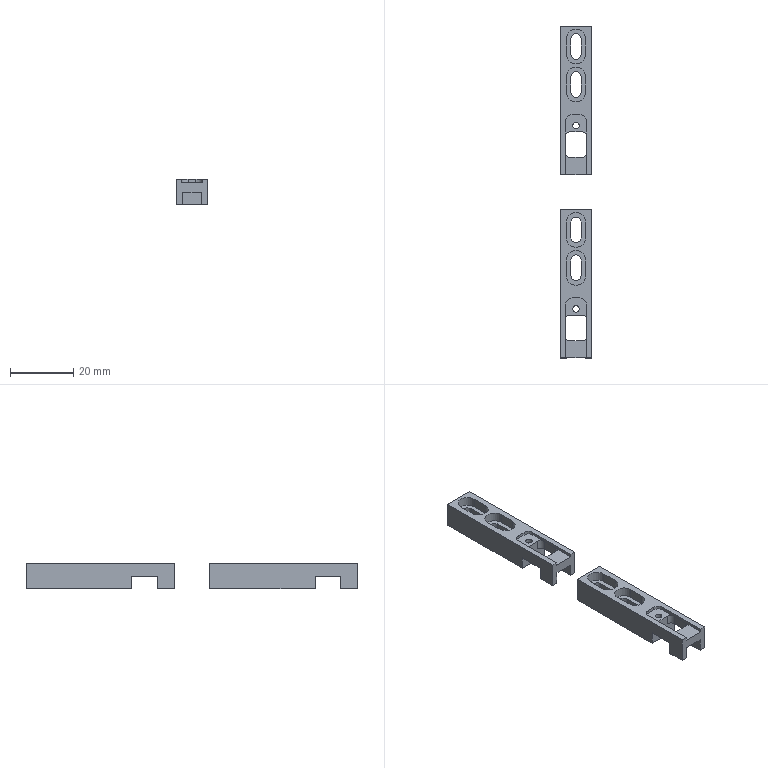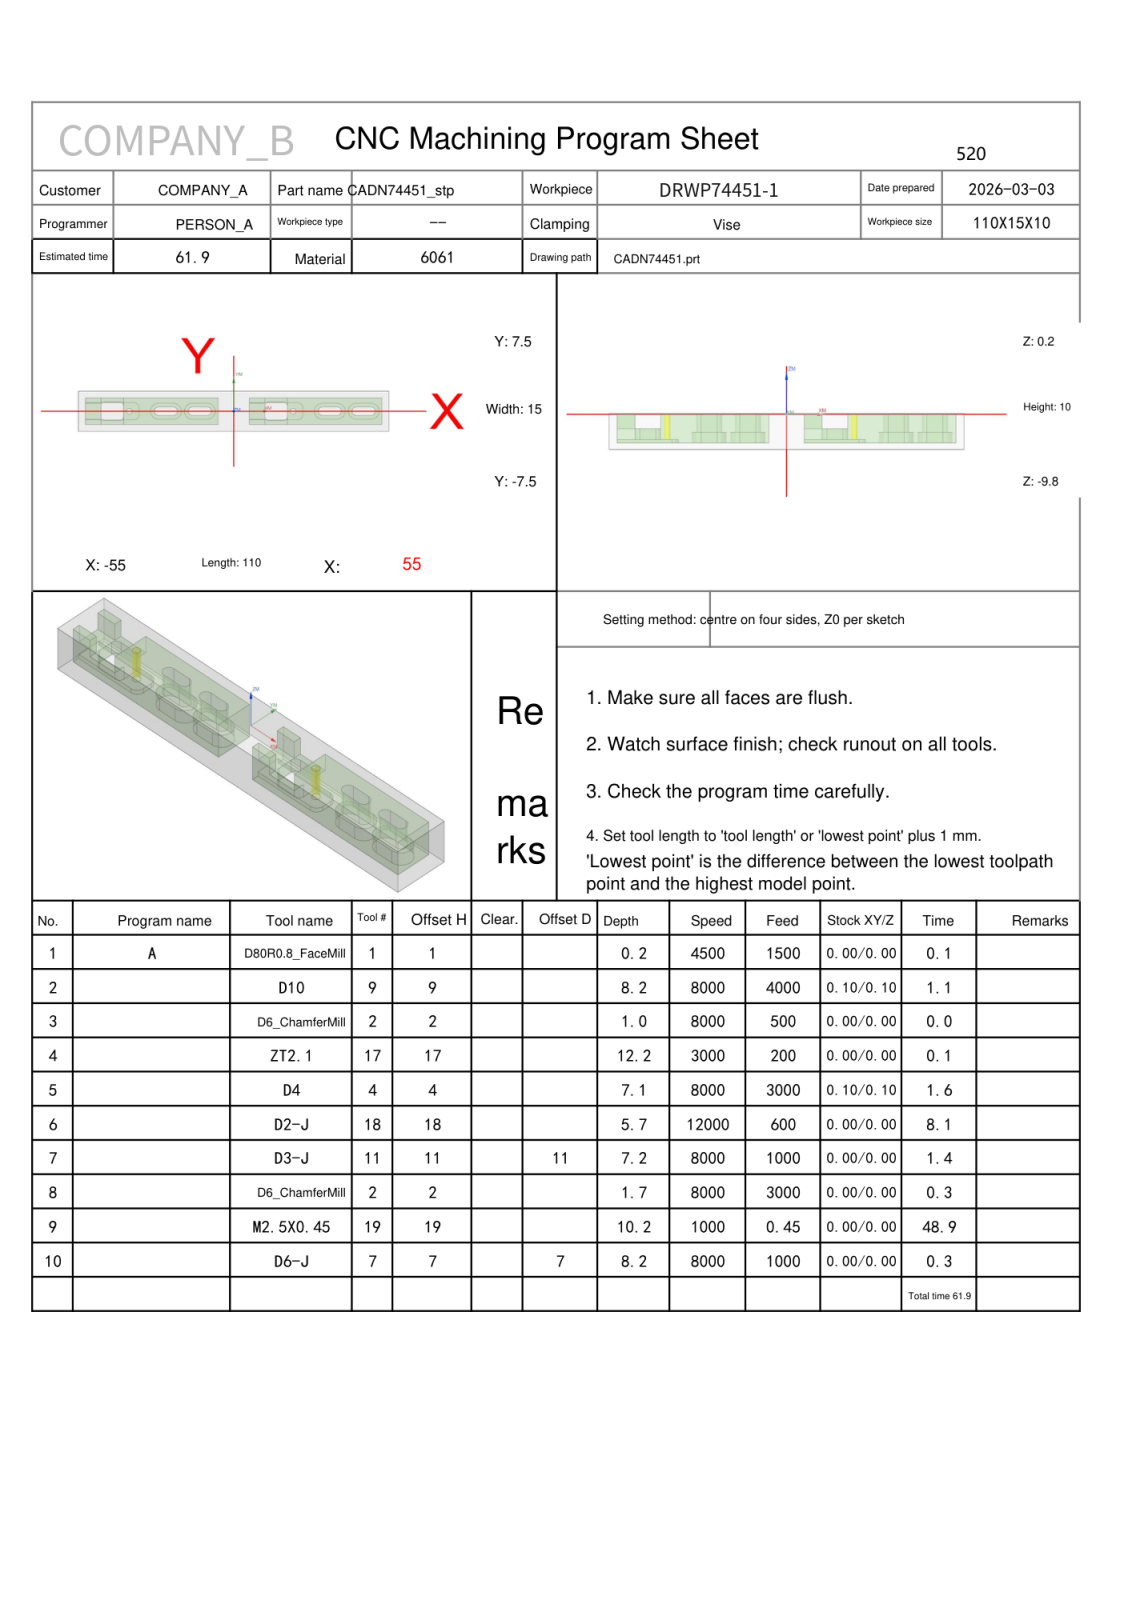NC program | NX | posted by the shop | part box 10 x 105 x 8 mm
Lines 2025 to 2969 of 4761:
N6 T18 M06
(D2-J  D=2. R=0. H=18 ce=0.10 di=0.10)
G00 G90 G54 X-12. Y.5 M03 S12000
G43 H18 Z50.
M08
Z.5
G01 X-14.5 Z.485 F600.
G03 X-15. Y0.0 Z.48 I0.0 J-.5
X-14.5 Y-.5 Z.475 I.5 J0.0
G01 X-9.5 Z.445
G03 X-9. Y0.0 Z.44 I0.0 J.5
X-9.5 Y.5 Z.435 I-.5 J0.0
G01 X-14.5 Z.405
G03 X-15. Y0.0 Z.4 I0.0 J-.5
X-14.5 Y-.5 Z.395 I.5 J0.0
G01 X-9.5 Z.365
G03 X-9. Y0.0 Z.36 I0.0 J.5
X-9.5 Y.5 Z.355 I-.5 J0.0
G01 X-14.5 Z.325
G03 X-15. Y0.0 Z.32 I0.0 J-.5
X-14.5 Y-.5 Z.315 I.5 J0.0
G01 X-9.5 Z.285
G03 X-9. Y0.0 Z.28 I0.0 J.5
X-9.5 Y.5 Z.275 I-.5 J0.0
G01 X-14.5 Z.245
G03 X-15. Y0.0 Z.24 I0.0 J-.5
X-14.5 Y-.5 Z.235 I.5 J0.0
G01 X-9.5 Z.205
G03 X-9. Y0.0 Z.2 I0.0 J.5
X-9.5 Y.5 Z.195 I-.5 J0.0
G01 X-14.5 Z.165
G03 X-15. Y0.0 Z.16 I0.0 J-.5
X-14.5 Y-.5 Z.155 I.5 J0.0
G01 X-9.5 Z.125
G03 X-9. Y0.0 Z.12 I0.0 J.5
X-9.5 Y.5 Z.115 I-.5 J0.0
G01 X-14.5 Z.085
G03 X-15. Y0.0 Z.08 I0.0 J-.5
X-14.5 Y-.5 Z.075 I.5 J0.0
G01 X-9.5 Z.045
G03 X-9. Y0.0 Z.04 I0.0 J.5
X-9.5 Y.5 Z.035 I-.5 J0.0
G01 X-14.5 Z.005
G03 X-15. Y0.0 Z0.0 I0.0 J-.5
X-14.5 Y-.5 Z-.005 I.5 J0.0
G01 X-9.5 Z-.035
G03 X-9. Y0.0 Z-.04 I0.0 J.5
X-9.5 Y.5 Z-.045 I-.5 J0.0
G01 X-14.5 Z-.075
G03 X-15. Y0.0 Z-.08 I0.0 J-.5
X-14.5 Y-.5 Z-.085 I.5 J0.0
G01 X-9.5 Z-.115
G03 X-9. Y0.0 Z-.12 I0.0 J.5
X-9.5 Y.5 Z-.125 I-.5 J0.0
G01 X-14.5 Z-.155
G03 X-15. Y0.0 Z-.16 I0.0 J-.5
X-14.5 Y-.5 Z-.165 I.5 J0.0
G01 X-9.5 Z-.195
G03 X-9. Y0.0 Z-.2 I0.0 J.5
X-9.5 Y.5 Z-.205 I-.5 J0.0
G01 X-14.5 Z-.235
G03 X-15. Y0.0 Z-.24 I0.0 J-.5
X-14.5 Y-.5 Z-.245 I.5 J0.0
G01 X-9.5 Z-.275
G03 X-9. Y0.0 Z-.28 I0.0 J.5
X-9.5 Y.5 Z-.285 I-.5 J0.0
G01 X-14.5 Z-.315
G03 X-15. Y0.0 Z-.32 I0.0 J-.5
X-14.5 Y-.5 Z-.325 I.5 J0.0
G01 X-9.5 Z-.355
G03 X-9. Y0.0 Z-.36 I0.0 J.5
X-9.5 Y.5 Z-.365 I-.5 J0.0
G01 X-14.5 Z-.395
G03 X-15. Y0.0 Z-.4 I0.0 J-.5
X-14.5 Y-.5 Z-.405 I.5 J0.0
G01 X-9.5 Z-.435
G03 X-9. Y0.0 Z-.44 I0.0 J.5
X-9.5 Y.5 Z-.445 I-.5 J0.0
G01 X-14.5 Z-.475
G03 X-15. Y0.0 Z-.48 I0.0 J-.5
X-14.5 Y-.5 Z-.485 I.5 J0.0
G01 X-9.5 Z-.515
G03 X-9. Y0.0 Z-.52 I0.0 J.5
X-9.5 Y.5 Z-.525 I-.5 J0.0
G01 X-14.5 Z-.555
G03 X-15. Y0.0 Z-.56 I0.0 J-.5
X-14.5 Y-.5 Z-.565 I.5 J0.0
G01 X-9.5 Z-.595
G03 X-9. Y0.0 Z-.6 I0.0 J.5
X-9.5 Y.5 Z-.605 I-.5 J0.0
G01 X-14.5 Z-.635
G03 X-15. Y0.0 Z-.64 I0.0 J-.5
X-14.5 Y-.5 Z-.645 I.5 J0.0
G01 X-9.5 Z-.675
G03 X-9. Y0.0 Z-.68 I0.0 J.5
X-9.5 Y.5 Z-.685 I-.5 J0.0
G01 X-14.5 Z-.715
G03 X-15. Y0.0 Z-.72 I0.0 J-.5
X-14.5 Y-.5 Z-.725 I.5 J0.0
G01 X-9.5 Z-.755
G03 X-9. Y0.0 Z-.76 I0.0 J.5
X-9.5 Y.5 Z-.765 I-.5 J0.0
G01 X-14.5 Z-.795
G03 X-15. Y0.0 Z-.8 I0.0 J-.5
X-14.5 Y-.5 Z-.805 I.5 J0.0
G01 X-9.5 Z-.835
G03 X-9. Y0.0 Z-.84 I0.0 J.5
X-9.5 Y.5 Z-.845 I-.5 J0.0
G01 X-14.5 Z-.875
G03 X-15. Y0.0 Z-.88 I0.0 J-.5
X-14.5 Y-.5 Z-.885 I.5 J0.0
G01 X-9.5 Z-.915
G03 X-9. Y0.0 Z-.92 I0.0 J.5
X-9.5 Y.5 Z-.925 I-.5 J0.0
G01 X-14.5 Z-.955
G03 X-15. Y0.0 Z-.96 I0.0 J-.5
X-14.5 Y-.5 Z-.965 I.5 J0.0
G01 X-9.5 Z-.995
G03 X-9. Y0.0 Z-1. I0.0 J.5
X-9.5 Y.5 Z-1.005 I-.5 J0.0
G01 X-14.5 Z-1.035
G03 X-15. Y0.0 Z-1.04 I0.0 J-.5
X-14.5 Y-.5 Z-1.045 I.5 J0.0
G01 X-9.5 Z-1.075
G03 X-9. Y0.0 Z-1.08 I0.0 J.5
X-9.5 Y.5 Z-1.085 I-.5 J0.0
G01 X-14.5 Z-1.115
G03 X-15. Y0.0 Z-1.12 I0.0 J-.5
X-14.5 Y-.5 Z-1.125 I.5 J0.0
G01 X-9.5 Z-1.155
G03 X-9. Y0.0 Z-1.16 I0.0 J.5
X-9.5 Y.5 Z-1.165 I-.5 J0.0
G01 X-14.5 Z-1.195
G03 X-15. Y0.0 Z-1.2 I0.0 J-.5
X-14.5 Y-.5 Z-1.205 I.5 J0.0
G01 X-9.5 Z-1.235
G03 X-9. Y0.0 Z-1.24 I0.0 J.5
X-9.5 Y.5 Z-1.245 I-.5 J0.0
G01 X-14.5 Z-1.275
G03 X-15. Y0.0 Z-1.28 I0.0 J-.5
X-14.5 Y-.5 Z-1.285 I.5 J0.0
G01 X-9.5 Z-1.315
G03 X-9. Y0.0 Z-1.32 I0.0 J.5
X-9.5 Y.5 Z-1.325 I-.5 J0.0
G01 X-14.5 Z-1.355
G03 X-15. Y0.0 Z-1.36 I0.0 J-.5
X-14.5 Y-.5 Z-1.365 I.5 J0.0
G01 X-9.5 Z-1.395
G03 X-9. Y0.0 Z-1.4 I0.0 J.5
X-9.5 Y.5 Z-1.405 I-.5 J0.0
G01 X-14.5 Z-1.435
G03 X-15. Y0.0 Z-1.44 I0.0 J-.5
X-14.5 Y-.5 Z-1.445 I.5 J0.0
G01 X-9.5 Z-1.475
G03 X-9. Y0.0 Z-1.48 I0.0 J.5
X-9.5 Y.5 Z-1.485 I-.5 J0.0
G01 X-14.5 Z-1.515
G03 X-15. Y0.0 Z-1.52 I0.0 J-.5
X-14.5 Y-.5 Z-1.525 I.5 J0.0
G01 X-9.5 Z-1.555
G03 X-9. Y0.0 Z-1.56 I0.0 J.5
X-9.5 Y.5 Z-1.565 I-.5 J0.0
G01 X-14.5 Z-1.595
G03 X-15. Y0.0 Z-1.6 I0.0 J-.5
X-14.5 Y-.5 Z-1.605 I.5 J0.0
G01 X-9.5 Z-1.635
G03 X-9. Y0.0 Z-1.64 I0.0 J.5
X-9.5 Y.5 Z-1.645 I-.5 J0.0
G01 X-14.5 Z-1.675
G03 X-15. Y0.0 Z-1.68 I0.0 J-.5
X-14.5 Y-.5 Z-1.685 I.5 J0.0
G01 X-9.5 Z-1.715
G03 X-9. Y0.0 Z-1.72 I0.0 J.5
X-9.5 Y.5 Z-1.725 I-.5 J0.0
G01 X-14.5 Z-1.755
G03 X-15. Y0.0 Z-1.76 I0.0 J-.5
X-14.5 Y-.5 Z-1.765 I.5 J0.0
G01 X-9.5 Z-1.795
G03 X-9. Y0.0 Z-1.8 I0.0 J.5
X-9.5 Y.5 Z-1.805 I-.5 J0.0
G01 X-14.5 Z-1.835
G03 X-15. Y0.0 Z-1.84 I0.0 J-.5
X-14.5 Y-.5 Z-1.845 I.5 J0.0
G01 X-9.5 Z-1.875
G03 X-9. Y0.0 Z-1.88 I0.0 J.5
X-9.5 Y.5 Z-1.885 I-.5 J0.0
G01 X-14.5 Z-1.915
G03 X-15. Y0.0 Z-1.92 I0.0 J-.5
X-14.5 Y-.5 Z-1.925 I.5 J0.0
G01 X-9.5 Z-1.955
G03 X-9. Y0.0 Z-1.96 I0.0 J.5
X-9.5 Y.5 Z-1.965 I-.5 J0.0
G01 X-14.5 Z-1.995
G03 X-15. Y0.0 Z-2. I0.0 J-.5
X-14.5 Y-.5 Z-2.005 I.5 J0.0
G01 X-9.5 Z-2.035
G03 X-9. Y0.0 Z-2.04 I0.0 J.5
X-9.5 Y.5 Z-2.045 I-.5 J0.0
G01 X-14.5 Z-2.075
G03 X-15. Y0.0 Z-2.08 I0.0 J-.5
X-14.5 Y-.5 Z-2.085 I.5 J0.0
G01 X-9.5 Z-2.115
G03 X-9. Y0.0 Z-2.12 I0.0 J.5
X-9.5 Y.5 Z-2.125 I-.5 J0.0
G01 X-14.5 Z-2.155
G03 X-15. Y0.0 Z-2.16 I0.0 J-.5
X-14.5 Y-.5 Z-2.165 I.5 J0.0
G01 X-9.5 Z-2.195
G03 X-9. Y0.0 Z-2.2 I0.0 J.5
X-9.5 Y.5 Z-2.205 I-.5 J0.0
G01 X-14.5 Z-2.235
G03 X-15. Y0.0 Z-2.24 I0.0 J-.5
X-14.5 Y-.5 Z-2.245 I.5 J0.0
G01 X-9.5 Z-2.275
G03 X-9. Y0.0 Z-2.28 I0.0 J.5
X-9.5 Y.5 Z-2.285 I-.5 J0.0
G01 X-14.5 Z-2.315
G03 X-15. Y0.0 Z-2.32 I0.0 J-.5
X-14.5 Y-.5 Z-2.325 I.5 J0.0
G01 X-9.5 Z-2.355
G03 X-9. Y0.0 Z-2.36 I0.0 J.5
X-9.5 Y.5 Z-2.365 I-.5 J0.0
G01 X-14.5 Z-2.395
G03 X-15. Y0.0 Z-2.4 I0.0 J-.5
X-14.5 Y-.5 Z-2.405 I.5 J0.0
G01 X-9.5 Z-2.435
G03 X-9. Y0.0 Z-2.44 I0.0 J.5
X-9.5 Y.5 Z-2.445 I-.5 J0.0
G01 X-14.5 Z-2.475
G03 X-15. Y0.0 Z-2.48 I0.0 J-.5
X-14.5 Y-.5 Z-2.485 I.5 J0.0
G01 X-9.5 Z-2.515
G03 X-9. Y0.0 Z-2.52 I0.0 J.5
X-9.5 Y.5 Z-2.525 I-.5 J0.0
G01 X-14.5 Z-2.555
G03 X-15. Y0.0 Z-2.56 I0.0 J-.5
X-14.5 Y-.5 Z-2.565 I.5 J0.0
G01 X-9.5 Z-2.595
G03 X-9. Y0.0 Z-2.6 I0.0 J.5
X-9.5 Y.5 Z-2.605 I-.5 J0.0
G01 X-14.5 Z-2.635
G03 X-15. Y0.0 Z-2.64 I0.0 J-.5
X-14.5 Y-.5 Z-2.645 I.5 J0.0
G01 X-9.5 Z-2.675
G03 X-9. Y0.0 Z-2.68 I0.0 J.5
X-9.5 Y.5 Z-2.685 I-.5 J0.0
G01 X-14.5 Z-2.715
G03 X-15. Y0.0 Z-2.72 I0.0 J-.5
X-14.5 Y-.5 Z-2.725 I.5 J0.0
G01 X-9.5 Z-2.755
G03 X-9. Y0.0 Z-2.76 I0.0 J.5
X-9.5 Y.5 Z-2.765 I-.5 J0.0
G01 X-14.5 Z-2.795
G03 X-15. Y0.0 Z-2.8 I0.0 J-.5
X-14.5 Y-.5 Z-2.805 I.5 J0.0
G01 X-9.5 Z-2.835
G03 X-9. Y0.0 Z-2.84 I0.0 J.5
X-9.5 Y.5 Z-2.845 I-.5 J0.0
G01 X-14.5 Z-2.875
G03 X-15. Y0.0 Z-2.88 I0.0 J-.5
X-14.5 Y-.5 Z-2.885 I.5 J0.0
G01 X-9.5 Z-2.915
G03 X-9. Y0.0 Z-2.92 I0.0 J.5
X-9.5 Y.5 Z-2.925 I-.5 J0.0
G01 X-14.5 Z-2.955
G03 X-15. Y0.0 Z-2.96 I0.0 J-.5
X-14.5 Y-.5 Z-2.965 I.5 J0.0
G01 X-9.5 Z-2.995
G03 X-9. Y0.0 Z-3. I0.0 J.5
X-9.5 Y.5 Z-3.005 I-.5 J0.0
G01 X-14.5 Z-3.035
G03 X-15. Y0.0 Z-3.04 I0.0 J-.5
X-14.5 Y-.5 Z-3.045 I.5 J0.0
G01 X-9.5 Z-3.075
G03 X-9. Y0.0 Z-3.08 I0.0 J.5
X-9.5 Y.5 Z-3.085 I-.5 J0.0
G01 X-14.5 Z-3.115
G03 X-15. Y0.0 Z-3.12 I0.0 J-.5
X-14.5 Y-.5 Z-3.125 I.5 J0.0
G01 X-9.5 Z-3.155
G03 X-9. Y0.0 Z-3.16 I0.0 J.5
X-9.5 Y.5 Z-3.165 I-.5 J0.0
G01 X-14.5 Z-3.195
G03 X-15. Y0.0 Z-3.2 I0.0 J-.5
X-14.5 Y-.5 Z-3.205 I.5 J0.0
G01 X-9.5 Z-3.235
G03 X-9. Y0.0 Z-3.24 I0.0 J.5
X-9.5 Y.5 Z-3.245 I-.5 J0.0
G01 X-14.5 Z-3.275
G03 X-15. Y0.0 Z-3.28 I0.0 J-.5
X-14.5 Y-.5 Z-3.285 I.5 J0.0
G01 X-9.5 Z-3.315
G03 X-9. Y0.0 Z-3.32 I0.0 J.5
X-9.5 Y.5 Z-3.325 I-.5 J0.0
G01 X-14.5 Z-3.355
G03 X-15. Y0.0 Z-3.36 I0.0 J-.5
X-14.5 Y-.5 Z-3.365 I.5 J0.0
G01 X-9.5 Z-3.395
G03 X-9. Y0.0 Z-3.4 I0.0 J.5
X-9.5 Y.5 Z-3.405 I-.5 J0.0
G01 X-14.5 Z-3.435
G03 X-15. Y0.0 Z-3.44 I0.0 J-.5
X-14.5 Y-.5 Z-3.445 I.5 J0.0
G01 X-9.5 Z-3.475
G03 X-9. Y0.0 Z-3.48 I0.0 J.5
X-9.5 Y.5 Z-3.485 I-.5 J0.0
G01 X-14.5 Z-3.515
G03 X-15. Y0.0 Z-3.52 I0.0 J-.5
X-14.5 Y-.5 Z-3.525 I.5 J0.0
G01 X-9.5 Z-3.555
G03 X-9. Y0.0 Z-3.56 I0.0 J.5
X-9.5 Y.5 Z-3.565 I-.5 J0.0
G01 X-14.5 Z-3.595
G03 X-15. Y0.0 Z-3.6 I0.0 J-.5
X-14.5 Y-.5 Z-3.605 I.5 J0.0
G01 X-9.5 Z-3.635
G03 X-9. Y0.0 Z-3.64 I0.0 J.5
X-9.5 Y.5 Z-3.645 I-.5 J0.0
G01 X-14.5 Z-3.675
G03 X-15. Y0.0 Z-3.68 I0.0 J-.5
X-14.5 Y-.5 Z-3.685 I.5 J0.0
G01 X-9.5 Z-3.715
G03 X-9. Y0.0 Z-3.72 I0.0 J.5
X-9.5 Y.5 Z-3.725 I-.5 J0.0
G01 X-14.5 Z-3.755
G03 X-15. Y0.0 Z-3.76 I0.0 J-.5
X-14.5 Y-.5 Z-3.765 I.5 J0.0
G01 X-9.5 Z-3.795
G03 X-9. Y0.0 Z-3.8 I0.0 J.5
X-9.5 Y.5 Z-3.805 I-.5 J0.0
G01 X-14.5 Z-3.835
G03 X-15. Y0.0 Z-3.84 I0.0 J-.5
X-14.5 Y-.5 Z-3.845 I.5 J0.0
G01 X-9.5 Z-3.875
G03 X-9. Y0.0 Z-3.88 I0.0 J.5
X-9.5 Y.5 Z-3.885 I-.5 J0.0
G01 X-14.5 Z-3.915
G03 X-15. Y0.0 Z-3.92 I0.0 J-.5
X-14.5 Y-.5 Z-3.925 I.5 J0.0
G01 X-9.5 Z-3.955
G03 X-9. Y0.0 Z-3.96 I0.0 J.5
X-9.5 Y.5 Z-3.965 I-.5 J0.0
G01 X-14.5 Z-3.995
G03 X-15. Y0.0 Z-4. I0.0 J-.5
X-14.5 Y-.5 Z-4.005 I.5 J0.0
G01 X-9.5 Z-4.035
G03 X-9. Y0.0 Z-4.04 I0.0 J.5
X-9.5 Y.5 Z-4.045 I-.5 J0.0
G01 X-14.5 Z-4.075
G03 X-15. Y0.0 Z-4.08 I0.0 J-.5
X-14.5 Y-.5 Z-4.085 I.5 J0.0
G01 X-9.5 Z-4.115
G03 X-9. Y0.0 Z-4.12 I0.0 J.5
X-9.5 Y.5 Z-4.125 I-.5 J0.0
G01 X-14.5 Z-4.155
G03 X-15. Y0.0 Z-4.16 I0.0 J-.5
X-14.5 Y-.5 Z-4.165 I.5 J0.0
G01 X-9.5 Z-4.195
G03 X-9. Y0.0 Z-4.2 I0.0 J.5
X-9.5 Y.5 Z-4.205 I-.5 J0.0
G01 X-14.5 Z-4.235
G03 X-15. Y0.0 Z-4.24 I0.0 J-.5
X-14.5 Y-.5 Z-4.245 I.5 J0.0
G01 X-9.5 Z-4.275
G03 X-9. Y0.0 Z-4.28 I0.0 J.5
X-9.5 Y.5 Z-4.285 I-.5 J0.0
G01 X-14.5 Z-4.315
G03 X-15. Y0.0 Z-4.32 I0.0 J-.5
X-14.5 Y-.5 Z-4.325 I.5 J0.0
G01 X-9.5 Z-4.355
G03 X-9. Y0.0 Z-4.36 I0.0 J.5
X-9.5 Y.5 Z-4.365 I-.5 J0.0
G01 X-14.5 Z-4.395
G03 X-15. Y0.0 Z-4.4 I0.0 J-.5
X-14.5 Y-.5 Z-4.405 I.5 J0.0
G01 X-9.5 Z-4.435
G03 X-9. Y0.0 Z-4.44 I0.0 J.5
X-9.5 Y.5 Z-4.445 I-.5 J0.0
G01 X-14.5 Z-4.475
G03 X-15. Y0.0 Z-4.48 I0.0 J-.5
X-14.5 Y-.5 Z-4.485 I.5 J0.0
G01 X-9.5 Z-4.515
G03 X-9. Y0.0 Z-4.52 I0.0 J.5
X-9.5 Y.5 Z-4.525 I-.5 J0.0
G01 X-14.5 Z-4.555
G03 X-15. Y0.0 Z-4.56 I0.0 J-.5
X-14.5 Y-.5 Z-4.565 I.5 J0.0
G01 X-9.5 Z-4.595
G03 X-9. Y0.0 Z-4.6 I0.0 J.5
X-9.5 Y.5 Z-4.605 I-.5 J0.0
G01 X-14.5 Z-4.635
G03 X-15. Y0.0 Z-4.64 I0.0 J-.5
X-14.5 Y-.5 Z-4.645 I.5 J0.0
G01 X-9.5 Z-4.675
G03 X-9. Y0.0 Z-4.68 I0.0 J.5
X-9.5 Y.5 Z-4.685 I-.5 J0.0
G01 X-14.5 Z-4.715
G03 X-15. Y0.0 Z-4.72 I0.0 J-.5
X-14.5 Y-.5 Z-4.725 I.5 J0.0
G01 X-9.5 Z-4.755
G03 X-9. Y0.0 Z-4.76 I0.0 J.5
X-9.5 Y.5 Z-4.765 I-.5 J0.0
G01 X-14.5 Z-4.795
G03 X-15. Y0.0 Z-4.8 I0.0 J-.5
X-14.5 Y-.5 Z-4.805 I.5 J0.0
G01 X-9.5 Z-4.835
G03 X-9. Y0.0 Z-4.84 I0.0 J.5
X-9.5 Y.5 Z-4.845 I-.5 J0.0
G01 X-14.5 Z-4.875
G03 X-15. Y0.0 Z-4.88 I0.0 J-.5
X-14.5 Y-.5 Z-4.885 I.5 J0.0
G01 X-9.5 Z-4.915
G03 X-9. Y0.0 Z-4.92 I0.0 J.5
X-9.5 Y.5 Z-4.925 I-.5 J0.0
G01 X-14.5 Z-4.955
G03 X-15. Y0.0 Z-4.96 I0.0 J-.5
X-14.5 Y-.5 Z-4.965 I.5 J0.0
G01 X-9.5 Z-4.995
G03 X-9. Y0.0 Z-5. I0.0 J.5
X-9.5 Y.5 Z-5.005 I-.5 J0.0
G01 X-14.5 Z-5.035
G03 X-15. Y0.0 Z-5.04 I0.0 J-.5
X-14.5 Y-.5 Z-5.045 I.5 J0.0
G01 X-9.5 Z-5.075
G03 X-9. Y0.0 Z-5.08 I0.0 J.5
X-9.5 Y.5 Z-5.085 I-.5 J0.0
G01 X-14.5 Z-5.115
G03 X-15. Y0.0 Z-5.12 I0.0 J-.5
X-14.5 Y-.5 Z-5.125 I.5 J0.0
G01 X-9.5 Z-5.155
G03 X-9. Y0.0 Z-5.16 I0.0 J.5
X-9.5 Y.5 Z-5.165 I-.5 J0.0
G01 X-14.5 Z-5.195
G03 X-15. Y0.0 Z-5.2 I0.0 J-.5
X-14.5 Y-.5 Z-5.205 I.5 J0.0
G01 X-9.5 Z-5.235
G03 X-9. Y0.0 Z-5.24 I0.0 J.5
X-9.5 Y.5 Z-5.245 I-.5 J0.0
G01 X-14.5 Z-5.275
G03 X-15. Y0.0 Z-5.28 I0.0 J-.5
X-14.5 Y-.5 Z-5.285 I.5 J0.0
G01 X-9.5 Z-5.315
G03 X-9. Y0.0 Z-5.32 I0.0 J.5
X-9.5 Y.5 Z-5.325 I-.5 J0.0
G01 X-14.5 Z-5.355
G03 X-15. Y0.0 Z-5.36 I0.0 J-.5
X-14.5 Y-.5 Z-5.365 I.5 J0.0
G01 X-9.5 Z-5.395
G03 X-9. Y0.0 Z-5.4 I0.0 J.5
X-9.5 Y.5 Z-5.405 I-.5 J0.0
G01 X-14.5 Z-5.435
G03 X-15. Y0.0 Z-5.44 I0.0 J-.5
X-14.5 Y-.5 Z-5.445 I.5 J0.0
G01 X-9.5 Z-5.475
G03 X-9. Y0.0 Z-5.48 I0.0 J.5
X-9.5 Y.5 Z-5.485 I-.5 J0.0
G01 X-12. Z-5.5
X-14.5
G03 X-15. Y0.0 I0.0 J-.5
X-14.5 Y-.5 I.5 J0.0
G01 X-9.5
G03 X-9. Y0.0 I0.0 J.5
X-9.5 Y.5 I-.5 J0.0
G01 X-12.
X-12.5
Z-4.5
G00 Z50.
X-24.
Z.5
G01 X-26.5 Z.485
G03 X-27. Y0.0 Z.48 I0.0 J-.5
X-26.5 Y-.5 Z.475 I.5 J0.0
G01 X-21.5 Z.445
G03 X-21. Y0.0 Z.44 I0.0 J.5
X-21.5 Y.5 Z.435 I-.5 J0.0
G01 X-26.5 Z.405
G03 X-27. Y0.0 Z.4 I0.0 J-.5
X-26.5 Y-.5 Z.395 I.5 J0.0
G01 X-21.5 Z.365
G03 X-21. Y0.0 Z.36 I0.0 J.5
X-21.5 Y.5 Z.355 I-.5 J0.0
G01 X-26.5 Z.325
G03 X-27. Y0.0 Z.32 I0.0 J-.5
X-26.5 Y-.5 Z.315 I.5 J0.0
G01 X-21.5 Z.285
G03 X-21. Y0.0 Z.28 I0.0 J.5
X-21.5 Y.5 Z.275 I-.5 J0.0
G01 X-26.5 Z.245
G03 X-27. Y0.0 Z.24 I0.0 J-.5
X-26.5 Y-.5 Z.235 I.5 J0.0
G01 X-21.5 Z.205
G03 X-21. Y0.0 Z.2 I0.0 J.5
X-21.5 Y.5 Z.195 I-.5 J0.0
G01 X-26.5 Z.165
G03 X-27. Y0.0 Z.16 I0.0 J-.5
X-26.5 Y-.5 Z.155 I.5 J0.0
G01 X-21.5 Z.125
G03 X-21. Y0.0 Z.12 I0.0 J.5
X-21.5 Y.5 Z.115 I-.5 J0.0
G01 X-26.5 Z.085
G03 X-27. Y0.0 Z.08 I0.0 J-.5
X-26.5 Y-.5 Z.075 I.5 J0.0
G01 X-21.5 Z.045
G03 X-21. Y0.0 Z.04 I0.0 J.5
X-21.5 Y.5 Z.035 I-.5 J0.0
G01 X-26.5 Z.005
G03 X-27. Y0.0 Z0.0 I0.0 J-.5
X-26.5 Y-.5 Z-.005 I.5 J0.0
G01 X-21.5 Z-.035
G03 X-21. Y0.0 Z-.04 I0.0 J.5
X-21.5 Y.5 Z-.045 I-.5 J0.0
G01 X-26.5 Z-.075
G03 X-27. Y0.0 Z-.08 I0.0 J-.5
X-26.5 Y-.5 Z-.085 I.5 J0.0
G01 X-21.5 Z-.115
G03 X-21. Y0.0 Z-.12 I0.0 J.5
X-21.5 Y.5 Z-.125 I-.5 J0.0
G01 X-26.5 Z-.155
G03 X-27. Y0.0 Z-.16 I0.0 J-.5
X-26.5 Y-.5 Z-.165 I.5 J0.0
G01 X-21.5 Z-.195
G03 X-21. Y0.0 Z-.2 I0.0 J.5
X-21.5 Y.5 Z-.205 I-.5 J0.0
G01 X-26.5 Z-.235
G03 X-27. Y0.0 Z-.24 I0.0 J-.5
X-26.5 Y-.5 Z-.245 I.5 J0.0
G01 X-21.5 Z-.275
G03 X-21. Y0.0 Z-.28 I0.0 J.5
X-21.5 Y.5 Z-.285 I-.5 J0.0
G01 X-26.5 Z-.315
G03 X-27. Y0.0 Z-.32 I0.0 J-.5
X-26.5 Y-.5 Z-.325 I.5 J0.0
G01 X-21.5 Z-.355
G03 X-21. Y0.0 Z-.36 I0.0 J.5
X-21.5 Y.5 Z-.365 I-.5 J0.0
G01 X-26.5 Z-.395
G03 X-27. Y0.0 Z-.4 I0.0 J-.5
X-26.5 Y-.5 Z-.405 I.5 J0.0
G01 X-21.5 Z-.435
G03 X-21. Y0.0 Z-.44 I0.0 J.5
X-21.5 Y.5 Z-.445 I-.5 J0.0
G01 X-26.5 Z-.475
G03 X-27. Y0.0 Z-.48 I0.0 J-.5
X-26.5 Y-.5 Z-.485 I.5 J0.0
G01 X-21.5 Z-.515
G03 X-21. Y0.0 Z-.52 I0.0 J.5
X-21.5 Y.5 Z-.525 I-.5 J0.0
G01 X-26.5 Z-.555
G03 X-27. Y0.0 Z-.56 I0.0 J-.5
X-26.5 Y-.5 Z-.565 I.5 J0.0
G01 X-21.5 Z-.595
G03 X-21. Y0.0 Z-.6 I0.0 J.5
X-21.5 Y.5 Z-.605 I-.5 J0.0
G01 X-26.5 Z-.635
G03 X-27. Y0.0 Z-.64 I0.0 J-.5
X-26.5 Y-.5 Z-.645 I.5 J0.0
G01 X-21.5 Z-.675
G03 X-21. Y0.0 Z-.68 I0.0 J.5
X-21.5 Y.5 Z-.685 I-.5 J0.0
G01 X-26.5 Z-.715
G03 X-27. Y0.0 Z-.72 I0.0 J-.5
X-26.5 Y-.5 Z-.725 I.5 J0.0
G01 X-21.5 Z-.755
G03 X-21. Y0.0 Z-.76 I0.0 J.5
X-21.5 Y.5 Z-.765 I-.5 J0.0
G01 X-26.5 Z-.795
G03 X-27. Y0.0 Z-.8 I0.0 J-.5
X-26.5 Y-.5 Z-.805 I.5 J0.0
G01 X-21.5 Z-.835
G03 X-21. Y0.0 Z-.84 I0.0 J.5
X-21.5 Y.5 Z-.845 I-.5 J0.0
G01 X-26.5 Z-.875
G03 X-27. Y0.0 Z-.88 I0.0 J-.5
X-26.5 Y-.5 Z-.885 I.5 J0.0
G01 X-21.5 Z-.915
G03 X-21. Y0.0 Z-.92 I0.0 J.5
X-21.5 Y.5 Z-.925 I-.5 J0.0
G01 X-26.5 Z-.955
G03 X-27. Y0.0 Z-.96 I0.0 J-.5
X-26.5 Y-.5 Z-.965 I.5 J0.0
G01 X-21.5 Z-.995
G03 X-21. Y0.0 Z-1. I0.0 J.5
X-21.5 Y.5 Z-1.005 I-.5 J0.0
G01 X-26.5 Z-1.035
G03 X-27. Y0.0 Z-1.04 I0.0 J-.5
X-26.5 Y-.5 Z-1.045 I.5 J0.0
G01 X-21.5 Z-1.075
G03 X-21. Y0.0 Z-1.08 I0.0 J.5
X-21.5 Y.5 Z-1.085 I-.5 J0.0
G01 X-26.5 Z-1.115
G03 X-27. Y0.0 Z-1.12 I0.0 J-.5
X-26.5 Y-.5 Z-1.125 I.5 J0.0
G01 X-21.5 Z-1.155
G03 X-21. Y0.0 Z-1.16 I0.0 J.5
X-21.5 Y.5 Z-1.165 I-.5 J0.0
G01 X-26.5 Z-1.195
G03 X-27. Y0.0 Z-1.2 I0.0 J-.5
X-26.5 Y-.5 Z-1.205 I.5 J0.0
G01 X-21.5 Z-1.235
G03 X-21. Y0.0 Z-1.24 I0.0 J.5
X-21.5 Y.5 Z-1.245 I-.5 J0.0
G01 X-26.5 Z-1.275
G03 X-27. Y0.0 Z-1.28 I0.0 J-.5
X-26.5 Y-.5 Z-1.285 I.5 J0.0
G01 X-21.5 Z-1.315
G03 X-21. Y0.0 Z-1.32 I0.0 J.5
X-21.5 Y.5 Z-1.325 I-.5 J0.0
G01 X-26.5 Z-1.355
G03 X-27. Y0.0 Z-1.36 I0.0 J-.5
X-26.5 Y-.5 Z-1.365 I.5 J0.0
G01 X-21.5 Z-1.395
G03 X-21. Y0.0 Z-1.4 I0.0 J.5
X-21.5 Y.5 Z-1.405 I-.5 J0.0
G01 X-26.5 Z-1.435
G03 X-27. Y0.0 Z-1.44 I0.0 J-.5
X-26.5 Y-.5 Z-1.445 I.5 J0.0
G01 X-21.5 Z-1.475
G03 X-21. Y0.0 Z-1.48 I0.0 J.5
X-21.5 Y.5 Z-1.485 I-.5 J0.0
G01 X-26.5 Z-1.515
G03 X-27. Y0.0 Z-1.52 I0.0 J-.5
X-26.5 Y-.5 Z-1.525 I.5 J0.0
G01 X-21.5 Z-1.555
G03 X-21. Y0.0 Z-1.56 I0.0 J.5
X-21.5 Y.5 Z-1.565 I-.5 J0.0
G01 X-26.5 Z-1.595
G03 X-27. Y0.0 Z-1.6 I0.0 J-.5
X-26.5 Y-.5 Z-1.605 I.5 J0.0
G01 X-21.5 Z-1.635
G03 X-21. Y0.0 Z-1.64 I0.0 J.5
X-21.5 Y.5 Z-1.645 I-.5 J0.0
G01 X-26.5 Z-1.675
G03 X-27. Y0.0 Z-1.68 I0.0 J-.5
X-26.5 Y-.5 Z-1.685 I.5 J0.0
G01 X-21.5 Z-1.715
G03 X-21. Y0.0 Z-1.72 I0.0 J.5
X-21.5 Y.5 Z-1.725 I-.5 J0.0
G01 X-26.5 Z-1.755
G03 X-27. Y0.0 Z-1.76 I0.0 J-.5
X-26.5 Y-.5 Z-1.765 I.5 J0.0
G01 X-21.5 Z-1.795
G03 X-21. Y0.0 Z-1.8 I0.0 J.5
X-21.5 Y.5 Z-1.805 I-.5 J0.0
G01 X-26.5 Z-1.835
G03 X-27. Y0.0 Z-1.84 I0.0 J-.5
X-26.5 Y-.5 Z-1.845 I.5 J0.0
G01 X-21.5 Z-1.875
G03 X-21. Y0.0 Z-1.88 I0.0 J.5
X-21.5 Y.5 Z-1.885 I-.5 J0.0
G01 X-26.5 Z-1.915
G03 X-27. Y0.0 Z-1.92 I0.0 J-.5
X-26.5 Y-.5 Z-1.925 I.5 J0.0
G01 X-21.5 Z-1.955
G03 X-21. Y0.0 Z-1.96 I0.0 J.5
X-21.5 Y.5 Z-1.965 I-.5 J0.0
G01 X-26.5 Z-1.995
G03 X-27. Y0.0 Z-2. I0.0 J-.5
X-26.5 Y-.5 Z-2.005 I.5 J0.0
G01 X-21.5 Z-2.035
G03 X-21. Y0.0 Z-2.04 I0.0 J.5
X-21.5 Y.5 Z-2.045 I-.5 J0.0
G01 X-26.5 Z-2.075
G03 X-27. Y0.0 Z-2.08 I0.0 J-.5
X-26.5 Y-.5 Z-2.085 I.5 J0.0
G01 X-21.5 Z-2.115
G03 X-21. Y0.0 Z-2.12 I0.0 J.5
X-21.5 Y.5 Z-2.125 I-.5 J0.0
G01 X-26.5 Z-2.155
G03 X-27. Y0.0 Z-2.16 I0.0 J-.5
X-26.5 Y-.5 Z-2.165 I.5 J0.0
G01 X-21.5 Z-2.195
G03 X-21. Y0.0 Z-2.2 I0.0 J.5
X-21.5 Y.5 Z-2.205 I-.5 J0.0
G01 X-26.5 Z-2.235
G03 X-27. Y0.0 Z-2.24 I0.0 J-.5
X-26.5 Y-.5 Z-2.245 I.5 J0.0
G01 X-21.5 Z-2.275
G03 X-21. Y0.0 Z-2.28 I0.0 J.5
X-21.5 Y.5 Z-2.285 I-.5 J0.0
G01 X-26.5 Z-2.315
G03 X-27. Y0.0 Z-2.32 I0.0 J-.5
X-26.5 Y-.5 Z-2.325 I.5 J0.0
G01 X-21.5 Z-2.355
G03 X-21. Y0.0 Z-2.36 I0.0 J.5
X-21.5 Y.5 Z-2.365 I-.5 J0.0
G01 X-26.5 Z-2.395
G03 X-27. Y0.0 Z-2.4 I0.0 J-.5
X-26.5 Y-.5 Z-2.405 I.5 J0.0
G01 X-21.5 Z-2.435
G03 X-21. Y0.0 Z-2.44 I0.0 J.5
X-21.5 Y.5 Z-2.445 I-.5 J0.0
G01 X-26.5 Z-2.475
G03 X-27. Y0.0 Z-2.48 I0.0 J-.5
X-26.5 Y-.5 Z-2.485 I.5 J0.0
G01 X-21.5 Z-2.515
G03 X-21. Y0.0 Z-2.52 I0.0 J.5
X-21.5 Y.5 Z-2.525 I-.5 J0.0
G01 X-26.5 Z-2.555
G03 X-27. Y0.0 Z-2.56 I0.0 J-.5
X-26.5 Y-.5 Z-2.565 I.5 J0.0
G01 X-21.5 Z-2.595
G03 X-21. Y0.0 Z-2.6 I0.0 J.5
X-21.5 Y.5 Z-2.605 I-.5 J0.0
G01 X-26.5 Z-2.635
G03 X-27. Y0.0 Z-2.64 I0.0 J-.5
X-26.5 Y-.5 Z-2.645 I.5 J0.0
G01 X-21.5 Z-2.675
G03 X-21. Y0.0 Z-2.68 I0.0 J.5
X-21.5 Y.5 Z-2.685 I-.5 J0.0
G01 X-26.5 Z-2.715
G03 X-27. Y0.0 Z-2.72 I0.0 J-.5
X-26.5 Y-.5 Z-2.725 I.5 J0.0
G01 X-21.5 Z-2.755
G03 X-21. Y0.0 Z-2.76 I0.0 J.5
X-21.5 Y.5 Z-2.765 I-.5 J0.0
G01 X-26.5 Z-2.795
G03 X-27. Y0.0 Z-2.8 I0.0 J-.5
X-26.5 Y-.5 Z-2.805 I.5 J0.0
G01 X-21.5 Z-2.835
G03 X-21. Y0.0 Z-2.84 I0.0 J.5
X-21.5 Y.5 Z-2.845 I-.5 J0.0
G01 X-26.5 Z-2.875
G03 X-27. Y0.0 Z-2.88 I0.0 J-.5
X-26.5 Y-.5 Z-2.885 I.5 J0.0
G01 X-21.5 Z-2.915
G03 X-21. Y0.0 Z-2.92 I0.0 J.5
X-21.5 Y.5 Z-2.925 I-.5 J0.0
G01 X-26.5 Z-2.955
G03 X-27. Y0.0 Z-2.96 I0.0 J-.5
X-26.5 Y-.5 Z-2.965 I.5 J0.0
G01 X-21.5 Z-2.995
G03 X-21. Y0.0 Z-3. I0.0 J.5
X-21.5 Y.5 Z-3.005 I-.5 J0.0
G01 X-26.5 Z-3.035
G03 X-27. Y0.0 Z-3.04 I0.0 J-.5
X-26.5 Y-.5 Z-3.045 I.5 J0.0
G01 X-21.5 Z-3.075
G03 X-21. Y0.0 Z-3.08 I0.0 J.5
X-21.5 Y.5 Z-3.085 I-.5 J0.0
G01 X-26.5 Z-3.115
G03 X-27. Y0.0 Z-3.12 I0.0 J-.5
X-26.5 Y-.5 Z-3.125 I.5 J0.0
G01 X-21.5 Z-3.155
G03 X-21. Y0.0 Z-3.16 I0.0 J.5
X-21.5 Y.5 Z-3.165 I-.5 J0.0
G01 X-26.5 Z-3.195
G03 X-27. Y0.0 Z-3.2 I0.0 J-.5
X-26.5 Y-.5 Z-3.205 I.5 J0.0
G01 X-21.5 Z-3.235
G03 X-21. Y0.0 Z-3.24 I0.0 J.5
X-21.5 Y.5 Z-3.245 I-.5 J0.0
G01 X-26.5 Z-3.275
G03 X-27. Y0.0 Z-3.28 I0.0 J-.5
X-26.5 Y-.5 Z-3.285 I.5 J0.0
G01 X-21.5 Z-3.315
G03 X-21. Y0.0 Z-3.32 I0.0 J.5
X-21.5 Y.5 Z-3.325 I-.5 J0.0
G01 X-26.5 Z-3.355
G03 X-27. Y0.0 Z-3.36 I0.0 J-.5
X-26.5 Y-.5 Z-3.365 I.5 J0.0
G01 X-21.5 Z-3.395
G03 X-21. Y0.0 Z-3.4 I0.0 J.5
X-21.5 Y.5 Z-3.405 I-.5 J0.0
G01 X-26.5 Z-3.435
G03 X-27. Y0.0 Z-3.44 I0.0 J-.5
X-26.5 Y-.5 Z-3.445 I.5 J0.0
G01 X-21.5 Z-3.475
G03 X-21. Y0.0 Z-3.48 I0.0 J.5
X-21.5 Y.5 Z-3.485 I-.5 J0.0
G01 X-26.5 Z-3.515
G03 X-27. Y0.0 Z-3.52 I0.0 J-.5
X-26.5 Y-.5 Z-3.525 I.5 J0.0
G01 X-21.5 Z-3.555
G03 X-21. Y0.0 Z-3.56 I0.0 J.5
X-21.5 Y.5 Z-3.565 I-.5 J0.0
G01 X-26.5 Z-3.595
G03 X-27. Y0.0 Z-3.6 I0.0 J-.5
X-26.5 Y-.5 Z-3.605 I.5 J0.0
G01 X-21.5 Z-3.635
G03 X-21. Y0.0 Z-3.64 I0.0 J.5
X-21.5 Y.5 Z-3.645 I-.5 J0.0
G01 X-26.5 Z-3.675
G03 X-27. Y0.0 Z-3.68 I0.0 J-.5
X-26.5 Y-.5 Z-3.685 I.5 J0.0
G01 X-21.5 Z-3.715
G03 X-21. Y0.0 Z-3.72 I0.0 J.5
X-21.5 Y.5 Z-3.725 I-.5 J0.0
G01 X-26.5 Z-3.755
G03 X-27. Y0.0 Z-3.76 I0.0 J-.5
X-26.5 Y-.5 Z-3.765 I.5 J0.0
G01 X-21.5 Z-3.795
G03 X-21. Y0.0 Z-3.8 I0.0 J.5
X-21.5 Y.5 Z-3.805 I-.5 J0.0
G01 X-26.5 Z-3.835
G03 X-27. Y0.0 Z-3.84 I0.0 J-.5
X-26.5 Y-.5 Z-3.845 I.5 J0.0
G01 X-21.5 Z-3.875
G03 X-21. Y0.0 Z-3.88 I0.0 J.5
X-21.5 Y.5 Z-3.885 I-.5 J0.0
G01 X-26.5 Z-3.915
G03 X-27. Y0.0 Z-3.92 I0.0 J-.5
X-26.5 Y-.5 Z-3.925 I.5 J0.0
G01 X-21.5 Z-3.955
G03 X-21. Y0.0 Z-3.96 I0.0 J.5
X-21.5 Y.5 Z-3.965 I-.5 J0.0
G01 X-26.5 Z-3.995
G03 X-27. Y0.0 Z-4. I0.0 J-.5
X-26.5 Y-.5 Z-4.005 I.5 J0.0
G01 X-21.5 Z-4.035
G03 X-21. Y0.0 Z-4.04 I0.0 J.5
X-21.5 Y.5 Z-4.045 I-.5 J0.0
G01 X-26.5 Z-4.075
G03 X-27. Y0.0 Z-4.08 I0.0 J-.5
X-26.5 Y-.5 Z-4.085 I.5 J0.0
G01 X-21.5 Z-4.115
G03 X-21. Y0.0 Z-4.12 I0.0 J.5
X-21.5 Y.5 Z-4.125 I-.5 J0.0
G01 X-26.5 Z-4.155
G03 X-27. Y0.0 Z-4.16 I0.0 J-.5
X-26.5 Y-.5 Z-4.165 I.5 J0.0
G01 X-21.5 Z-4.195
G03 X-21. Y0.0 Z-4.2 I0.0 J.5
X-21.5 Y.5 Z-4.205 I-.5 J0.0
G01 X-26.5 Z-4.235
G03 X-27. Y0.0 Z-4.24 I0.0 J-.5
X-26.5 Y-.5 Z-4.245 I.5 J0.0
G01 X-21.5 Z-4.275
G03 X-21. Y0.0 Z-4.28 I0.0 J.5
X-21.5 Y.5 Z-4.285 I-.5 J0.0
G01 X-26.5 Z-4.315
G03 X-27. Y0.0 Z-4.32 I0.0 J-.5
X-26.5 Y-.5 Z-4.325 I.5 J0.0
G01 X-21.5 Z-4.355
G03 X-21. Y0.0 Z-4.36 I0.0 J.5
X-21.5 Y.5 Z-4.365 I-.5 J0.0
G01 X-26.5 Z-4.395
G03 X-27. Y0.0 Z-4.4 I0.0 J-.5
X-26.5 Y-.5 Z-4.405 I.5 J0.0
G01 X-21.5 Z-4.435
G03 X-21. Y0.0 Z-4.44 I0.0 J.5
X-21.5 Y.5 Z-4.445 I-.5 J0.0
G01 X-26.5 Z-4.475
G03 X-27. Y0.0 Z-4.48 I0.0 J-.5
X-26.5 Y-.5 Z-4.485 I.5 J0.0
G01 X-21.5 Z-4.515
G03 X-21. Y0.0 Z-4.52 I0.0 J.5
X-21.5 Y.5 Z-4.525 I-.5 J0.0
G01 X-26.5 Z-4.555
G03 X-27. Y0.0 Z-4.56 I0.0 J-.5
X-26.5 Y-.5 Z-4.565 I.5 J0.0
G01 X-21.5 Z-4.595
G03 X-21. Y0.0 Z-4.6 I0.0 J.5
X-21.5 Y.5 Z-4.605 I-.5 J0.0
G01 X-26.5 Z-4.635
G03 X-27. Y0.0 Z-4.64 I0.0 J-.5
X-26.5 Y-.5 Z-4.645 I.5 J0.0
G01 X-21.5 Z-4.675
G03 X-21. Y0.0 Z-4.68 I0.0 J.5
X-21.5 Y.5 Z-4.685 I-.5 J0.0
G01 X-26.5 Z-4.715
G03 X-27. Y0.0 Z-4.72 I0.0 J-.5
X-26.5 Y-.5 Z-4.725 I.5 J0.0
G01 X-21.5 Z-4.755
G03 X-21. Y0.0 Z-4.76 I0.0 J.5
X-21.5 Y.5 Z-4.765 I-.5 J0.0
G01 X-26.5 Z-4.795
G03 X-27. Y0.0 Z-4.8 I0.0 J-.5
X-26.5 Y-.5 Z-4.805 I.5 J0.0
G01 X-21.5 Z-4.835
G03 X-21. Y0.0 Z-4.84 I0.0 J.5
X-21.5 Y.5 Z-4.845 I-.5 J0.0
G01 X-26.5 Z-4.875
G03 X-27. Y0.0 Z-4.88 I0.0 J-.5
X-26.5 Y-.5 Z-4.885 I.5 J0.0
G01 X-21.5 Z-4.915
G03 X-21. Y0.0 Z-4.92 I0.0 J.5
X-21.5 Y.5 Z-4.925 I-.5 J0.0
G01 X-26.5 Z-4.955
G03 X-27. Y0.0 Z-4.96 I0.0 J-.5
X-26.5 Y-.5 Z-4.965 I.5 J0.0
G01 X-21.5 Z-4.995
G03 X-21. Y0.0 Z-5. I0.0 J.5
X-21.5 Y.5 Z-5.005 I-.5 J0.0
G01 X-26.5 Z-5.035
G03 X-27. Y0.0 Z-5.04 I0.0 J-.5
X-26.5 Y-.5 Z-5.045 I.5 J0.0
G01 X-21.5 Z-5.075
G03 X-21. Y0.0 Z-5.08 I0.0 J.5
X-21.5 Y.5 Z-5.085 I-.5 J0.0
G01 X-26.5 Z-5.115
G03 X-27. Y0.0 Z-5.12 I0.0 J-.5
X-26.5 Y-.5 Z-5.125 I.5 J0.0
G01 X-21.5 Z-5.155
G03 X-21. Y0.0 Z-5.16 I0.0 J.5
X-21.5 Y.5 Z-5.165 I-.5 J0.0
G01 X-26.5 Z-5.195
G03 X-27. Y0.0 Z-5.2 I0.0 J-.5
X-26.5 Y-.5 Z-5.205 I.5 J0.0
G01 X-21.5 Z-5.235
G03 X-21. Y0.0 Z-5.24 I0.0 J.5
X-21.5 Y.5 Z-5.245 I-.5 J0.0
G01 X-26.5 Z-5.275
G03 X-27. Y0.0 Z-5.28 I0.0 J-.5
X-26.5 Y-.5 Z-5.285 I.5 J0.0
G01 X-21.5 Z-5.315
G03 X-21. Y0.0 Z-5.32 I0.0 J.5
X-21.5 Y.5 Z-5.325 I-.5 J0.0
G01 X-26.5 Z-5.355
G03 X-27. Y0.0 Z-5.36 I0.0 J-.5
X-26.5 Y-.5 Z-5.365 I.5 J0.0
G01 X-21.5 Z-5.395
G03 X-21. Y0.0 Z-5.4 I0.0 J.5
X-21.5 Y.5 Z-5.405 I-.5 J0.0
G01 X-26.5 Z-5.435
G03 X-27. Y0.0 Z-5.44 I0.0 J-.5
X-26.5 Y-.5 Z-5.445 I.5 J0.0
G01 X-21.5 Z-5.475
G03 X-21. Y0.0 Z-5.48 I0.0 J.5
X-21.5 Y.5 Z-5.485 I-.5 J0.0
G01 X-24. Z-5.5
X-26.5
G03 X-27. Y0.0 I0.0 J-.5
X-26.5 Y-.5 I.5 J0.0
G01 X-21.5
G03 X-21. Y0.0 I0.0 J.5
X-21.5 Y.5 I-.5 J0.0
G01 X-24.
X-24.5
Z-4.5
G00 Z50.
X46.
Z.5
G01 X43.5 Z.485
G03 X43. Y0.0 Z.48 I0.0 J-.5
X43.5 Y-.5 Z.475 I.5 J0.0
G01 X48.5 Z.445
G03 X49. Y0.0 Z.44 I0.0 J.5
X48.5 Y.5 Z.435 I-.5 J0.0
G01 X43.5 Z.405
G03 X43. Y0.0 Z.4 I0.0 J-.5
X43.5 Y-.5 Z.395 I.5 J0.0
G01 X48.5 Z.365
G03 X49. Y0.0 Z.36 I0.0 J.5
X48.5 Y.5 Z.355 I-.5 J0.0
G01 X43.5 Z.325